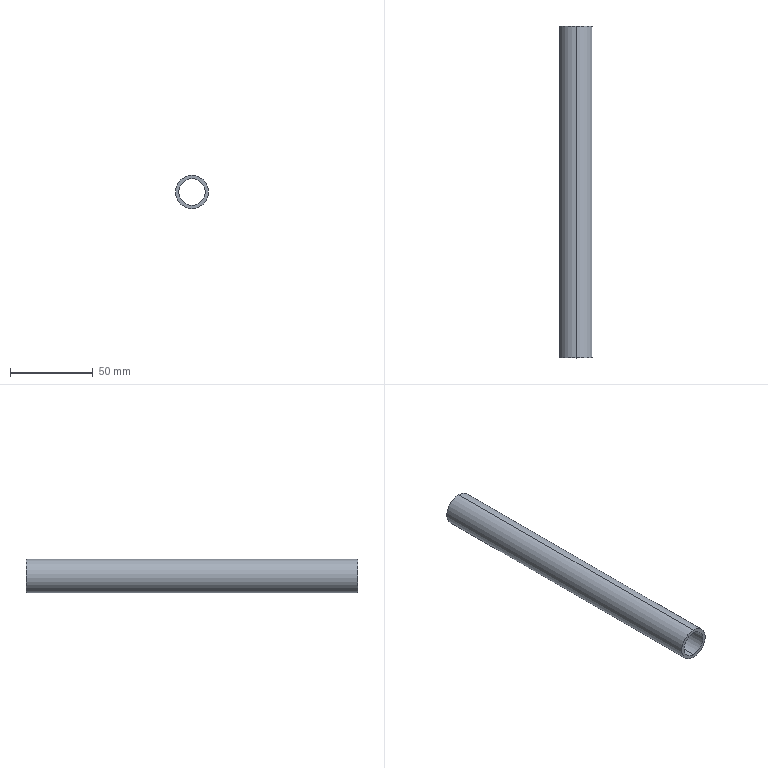Part | SolidWorks | features WeldMemberFeat 1, WeldmentFeature 1 | 1 solid | 6 faces | box 20 x 200 x 20 mm | volume 22619 mm3 | cylinder 4 | plane 2 | commonest cylinder face diameters 16 x2 20 x2
STEP:
#1=CARTESIAN_POINT('',(0.,200.,10.));
#2=VERTEX_POINT('',#1);
#3=CARTESIAN_POINT('',(0.,200.,-10.));
#4=VERTEX_POINT('',#3);
#5=CARTESIAN_POINT('',(0.,200.,0.));
#6=DIRECTION('',(0.,1.,0.));
#7=DIRECTION('',(0.,0.,1.));
#8=AXIS2_PLACEMENT_3D('',#5,#6,#7);
#9=CIRCLE('',#8,10.);
#10=EDGE_CURVE('',#2,#4,#9,.T.);
#11=ORIENTED_EDGE('',*,*,#10,.F.);
#12=CARTESIAN_POINT('',(0.,0.,10.));
#13=VERTEX_POINT('',#12);
#14=CARTESIAN_POINT('',(0.,200.,10.));
#15=DIRECTION('',(0.,-1.,0.));
#16=VECTOR('',#15,1000.);
#17=LINE('',#14,#16);
#18=EDGE_CURVE('',#2,#13,#17,.T.);
#19=ORIENTED_EDGE('',*,*,#18,.T.);
#20=CARTESIAN_POINT('',(0.,0.,-10.));
#21=VERTEX_POINT('',#20);
#22=CARTESIAN_POINT('',(0.,0.,0.));
#23=DIRECTION('',(0.,1.,0.));
#24=DIRECTION('',(0.,0.,1.));
#25=AXIS2_PLACEMENT_3D('',#22,#23,#24);
#26=CIRCLE('',#25,10.);
#27=EDGE_CURVE('',#13,#21,#26,.T.);
#28=ORIENTED_EDGE('',*,*,#27,.T.);
#29=CARTESIAN_POINT('',(0.,200.,-10.));
#30=DIRECTION('',(0.,-1.,0.));
#31=VECTOR('',#30,1000.);
#32=LINE('',#29,#31);
#33=EDGE_CURVE('',#4,#21,#32,.T.);
#34=ORIENTED_EDGE('',*,*,#33,.F.);
#35=EDGE_LOOP('',(#11,#19,#28,#34));
#36=FACE_OUTER_BOUND('',#35,.T.);
#37=CARTESIAN_POINT('',(0.,200.,0.));
#38=DIRECTION('',(0.,-1.,0.));
#39=DIRECTION('',(0.,0.,-1.));
#40=AXIS2_PLACEMENT_3D('',#37,#38,#39);
#41=CYLINDRICAL_SURFACE('',#40,10.);
#42=ADVANCED_FACE('',(#36),#41,.T.);
#43=CARTESIAN_POINT('',(0.,200.,-8.));
#44=VERTEX_POINT('',#43);
#45=CARTESIAN_POINT('',(0.,200.,8.));
#46=VERTEX_POINT('',#45);
#47=CARTESIAN_POINT('',(0.,200.,0.));
#48=DIRECTION('',(0.,1.,0.));
#49=DIRECTION('',(0.,0.,1.));
#50=AXIS2_PLACEMENT_3D('',#47,#48,#49);
#51=CIRCLE('',#50,8.);
#52=EDGE_CURVE('',#44,#46,#51,.T.);
#53=ORIENTED_EDGE('',*,*,#52,.T.);
#54=CARTESIAN_POINT('',(0.,0.,8.));
#55=VERTEX_POINT('',#54);
#56=CARTESIAN_POINT('',(0.,200.,8.));
#57=DIRECTION('',(0.,-1.,0.));
#58=VECTOR('',#57,1000.);
#59=LINE('',#56,#58);
#60=EDGE_CURVE('',#46,#55,#59,.T.);
#61=ORIENTED_EDGE('',*,*,#60,.T.);
#62=CARTESIAN_POINT('',(0.,0.,-8.));
#63=VERTEX_POINT('',#62);
#64=CARTESIAN_POINT('',(0.,0.,0.));
#65=DIRECTION('',(0.,1.,0.));
#66=DIRECTION('',(0.,0.,1.));
#67=AXIS2_PLACEMENT_3D('',#64,#65,#66);
#68=CIRCLE('',#67,8.);
#69=EDGE_CURVE('',#63,#55,#68,.T.);
#70=ORIENTED_EDGE('',*,*,#69,.F.);
#71=CARTESIAN_POINT('',(0.,200.,-8.));
#72=DIRECTION('',(0.,-1.,0.));
#73=VECTOR('',#72,1000.);
#74=LINE('',#71,#73);
#75=EDGE_CURVE('',#44,#63,#74,.T.);
#76=ORIENTED_EDGE('',*,*,#75,.F.);
#77=EDGE_LOOP('',(#53,#61,#70,#76));
#78=FACE_OUTER_BOUND('',#77,.T.);
#79=CARTESIAN_POINT('',(0.,200.,0.));
#80=DIRECTION('',(0.,-1.,0.));
#81=DIRECTION('',(0.,0.,-1.));
#82=AXIS2_PLACEMENT_3D('',#79,#80,#81);
#83=CYLINDRICAL_SURFACE('',#82,8.);
#84=ADVANCED_FACE('',(#78),#83,.F.);
#85=ORIENTED_EDGE('',*,*,#60,.F.);
#86=CARTESIAN_POINT('',(0.,200.,0.));
#87=DIRECTION('',(0.,1.,0.));
#88=DIRECTION('',(0.,0.,1.));
#89=AXIS2_PLACEMENT_3D('',#86,#87,#88);
#90=CIRCLE('',#89,8.);
#91=EDGE_CURVE('',#46,#44,#90,.T.);
#92=ORIENTED_EDGE('',*,*,#91,.T.);
#93=ORIENTED_EDGE('',*,*,#75,.T.);
#94=CARTESIAN_POINT('',(0.,0.,0.));
#95=DIRECTION('',(0.,1.,0.));
#96=DIRECTION('',(0.,0.,1.));
#97=AXIS2_PLACEMENT_3D('',#94,#95,#96);
#98=CIRCLE('',#97,8.);
#99=EDGE_CURVE('',#55,#63,#98,.T.);
#100=ORIENTED_EDGE('',*,*,#99,.F.);
#101=EDGE_LOOP('',(#85,#92,#93,#100));
#102=FACE_OUTER_BOUND('',#101,.T.);
#103=CARTESIAN_POINT('',(0.,200.,0.));
#104=DIRECTION('',(0.,-1.,0.));
#105=DIRECTION('',(0.,0.,-1.));
#106=AXIS2_PLACEMENT_3D('',#103,#104,#105);
#107=CYLINDRICAL_SURFACE('',#106,8.);
#108=ADVANCED_FACE('',(#102),#107,.F.);
#109=ORIENTED_EDGE('',*,*,#18,.F.);
#110=CARTESIAN_POINT('',(0.,200.,0.));
#111=DIRECTION('',(0.,1.,0.));
#112=DIRECTION('',(0.,0.,1.));
#113=AXIS2_PLACEMENT_3D('',#110,#111,#112);
#114=CIRCLE('',#113,10.);
#115=EDGE_CURVE('',#4,#2,#114,.T.);
#116=ORIENTED_EDGE('',*,*,#115,.F.);
#117=ORIENTED_EDGE('',*,*,#33,.T.);
#118=CARTESIAN_POINT('',(0.,0.,0.));
#119=DIRECTION('',(0.,1.,0.));
#120=DIRECTION('',(0.,0.,1.));
#121=AXIS2_PLACEMENT_3D('',#118,#119,#120);
#122=CIRCLE('',#121,10.);
#123=EDGE_CURVE('',#21,#13,#122,.T.);
#124=ORIENTED_EDGE('',*,*,#123,.T.);
#125=EDGE_LOOP('',(#109,#116,#117,#124));
#126=FACE_OUTER_BOUND('',#125,.T.);
#127=CARTESIAN_POINT('',(0.,200.,0.));
#128=DIRECTION('',(0.,-1.,0.));
#129=DIRECTION('',(0.,0.,-1.));
#130=AXIS2_PLACEMENT_3D('',#127,#128,#129);
#131=CYLINDRICAL_SURFACE('',#130,10.);
#132=ADVANCED_FACE('',(#126),#131,.T.);
#133=ORIENTED_EDGE('',*,*,#52,.F.);
#134=ORIENTED_EDGE('',*,*,#91,.F.);
#135=EDGE_LOOP('',(#133,#134));
#136=FACE_BOUND('',#135,.T.);
#137=ORIENTED_EDGE('',*,*,#115,.T.);
#138=ORIENTED_EDGE('',*,*,#10,.T.);
#139=EDGE_LOOP('',(#137,#138));
#140=FACE_OUTER_BOUND('',#139,.T.);
#141=CARTESIAN_POINT('',(0.,200.,0.));
#142=DIRECTION('',(0.,1.,0.));
#143=DIRECTION('',(0.,0.,1.));
#144=AXIS2_PLACEMENT_3D('',#141,#142,#143);
#145=PLANE('',#144);
#146=ADVANCED_FACE('',(#136,#140),#145,.T.);
#147=ORIENTED_EDGE('',*,*,#69,.T.);
#148=ORIENTED_EDGE('',*,*,#99,.T.);
#149=EDGE_LOOP('',(#147,#148));
#150=FACE_BOUND('',#149,.T.);
#151=ORIENTED_EDGE('',*,*,#123,.F.);
#152=ORIENTED_EDGE('',*,*,#27,.F.);
#153=EDGE_LOOP('',(#151,#152));
#154=FACE_OUTER_BOUND('',#153,.T.);
#155=CARTESIAN_POINT('',(0.,0.,0.));
#156=DIRECTION('',(0.,1.,0.));
#157=DIRECTION('',(0.,0.,1.));
#158=AXIS2_PLACEMENT_3D('',#155,#156,#157);
#159=PLANE('',#158);
#160=ADVANCED_FACE('',(#150,#154),#159,.F.);
#161=CLOSED_SHELL('',(#42,#84,#108,#132,#146,#160));
#162=MANIFOLD_SOLID_BREP('',#161);
#163=CARTESIAN_POINT('',(0.,0.,0.));
#164=DIRECTION('',(0.,0.,1.));
#165=DIRECTION('',(1.,0.,0.));
#166=AXIS2_PLACEMENT_3D('',#163,#164,#165);
#167=(LENGTH_UNIT()NAMED_UNIT(*)SI_UNIT(.MILLI.,.METRE.));
#168=UNCERTAINTY_MEASURE_WITH_UNIT(LENGTH_MEASURE(0.00001),#167,'','');
#169=(NAMED_UNIT(*)PLANE_ANGLE_UNIT()SI_UNIT($,.RADIAN.));
#170=(NAMED_UNIT(*)SI_UNIT($,.STERADIAN.)SOLID_ANGLE_UNIT());
#171=(GEOMETRIC_REPRESENTATION_CONTEXT(3)GLOBAL_UNCERTAINTY_ASSIGNED_CONTEXT((#168))GLOBAL_UNIT_ASSIGNED_CONTEXT((#167,#169,#170))REPRESENTATION_CONTEXT('',''));
#172=ADVANCED_BREP_SHAPE_REPRESENTATION('',(#162,#166),#171);